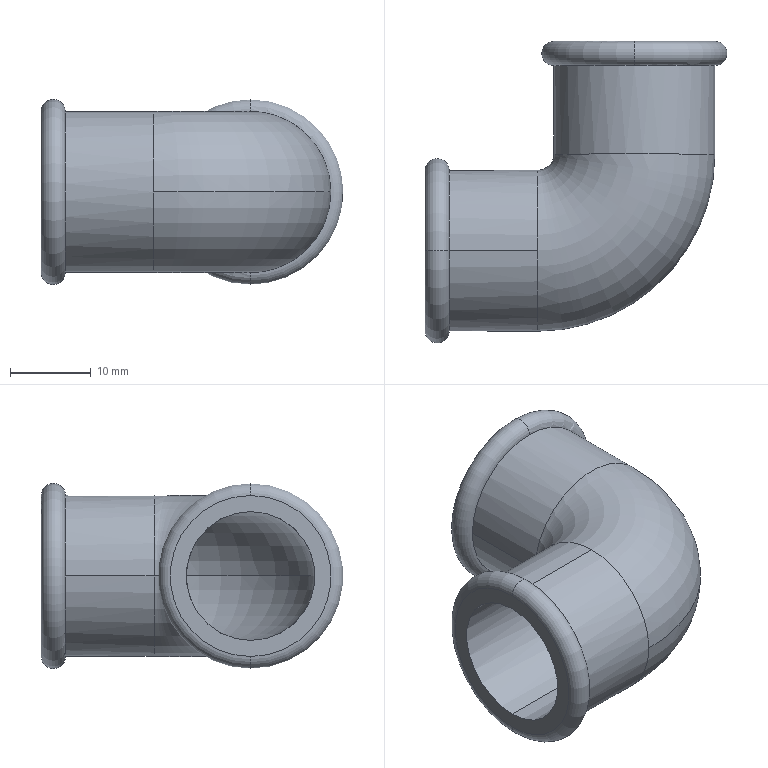Part | NX | features BREP 1 | 1 solid | 18 faces | box 37.5 x 37.5 x 23 mm | volume 5771 mm3 | torus 8 | cylinder 8 | plane 2 | commonest cylinder face diameters 16 x4 20 x4
STEP:
#1=CARTESIAN_POINT('',(34.,12.,0.));
#2=VERTEX_POINT('',#1);
#3=CARTESIAN_POINT('',(18.,12.,0.));
#4=VERTEX_POINT('',#3);
#5=CARTESIAN_POINT('',(26.,12.,0.));
#6=DIRECTION('',(0.,-1.,0.));
#7=DIRECTION('',(0.,0.,1.));
#8=AXIS2_PLACEMENT_3D('',#5,#6,#7);
#9=CIRCLE('',#8,8.);
#10=EDGE_CURVE('',#2,#4,#9,.T.);
#11=ORIENTED_EDGE('',*,*,#10,.F.);
#12=CARTESIAN_POINT('',(14.,-8.,0.));
#13=VERTEX_POINT('',#12);
#14=CARTESIAN_POINT('',(14.,12.,0.));
#15=DIRECTION('',(0.,0.,-1.));
#16=DIRECTION('',(-1.,0.,0.));
#17=AXIS2_PLACEMENT_3D('',#14,#15,#16);
#18=CIRCLE('',#17,20.);
#19=EDGE_CURVE('',#2,#13,#18,.T.);
#20=ORIENTED_EDGE('',*,*,#19,.T.);
#21=CARTESIAN_POINT('',(14.,0.,8.));
#22=VERTEX_POINT('',#21);
#23=CARTESIAN_POINT('',(14.,0.,0.));
#24=DIRECTION('',(-1.,0.,0.));
#25=DIRECTION('',(0.,0.,1.));
#26=AXIS2_PLACEMENT_3D('',#23,#24,#25);
#27=CIRCLE('',#26,8.);
#28=EDGE_CURVE('',#13,#22,#27,.T.);
#29=ORIENTED_EDGE('',*,*,#28,.T.);
#30=CARTESIAN_POINT('',(14.,8.,0.));
#31=VERTEX_POINT('',#30);
#32=CARTESIAN_POINT('',(14.,0.,0.));
#33=DIRECTION('',(-1.,0.,0.));
#34=DIRECTION('',(0.,0.,1.));
#35=AXIS2_PLACEMENT_3D('',#32,#33,#34);
#36=CIRCLE('',#35,8.);
#37=EDGE_CURVE('',#22,#31,#36,.T.);
#38=ORIENTED_EDGE('',*,*,#37,.T.);
#39=CARTESIAN_POINT('',(14.,12.,0.));
#40=DIRECTION('',(0.,0.,-1.));
#41=DIRECTION('',(-1.,0.,0.));
#42=AXIS2_PLACEMENT_3D('',#39,#40,#41);
#43=CIRCLE('',#42,4.);
#44=EDGE_CURVE('',#4,#31,#43,.T.);
#45=ORIENTED_EDGE('',*,*,#44,.F.);
#46=EDGE_LOOP('',(#11,#20,#29,#38,#45));
#47=FACE_BOUND('',#46,.T.);
#48=CARTESIAN_POINT('',(14.,12.,0.));
#49=DIRECTION('',(0.,0.,-1.));
#50=DIRECTION('',(-1.,0.,0.));
#51=AXIS2_PLACEMENT_3D('',#48,#49,#50);
#52=TOROIDAL_SURFACE('',#51,12.,8.);
#53=ADVANCED_FACE('',(#47),#52,.F.);
#54=CARTESIAN_POINT('',(16.,12.,0.));
#55=VERTEX_POINT('',#54);
#56=CARTESIAN_POINT('',(36.,12.,0.));
#57=VERTEX_POINT('',#56);
#58=CARTESIAN_POINT('',(26.,12.,0.));
#59=DIRECTION('',(0.,-1.,0.));
#60=DIRECTION('',(0.,0.,1.));
#61=AXIS2_PLACEMENT_3D('',#58,#59,#60);
#62=CIRCLE('',#61,10.);
#63=EDGE_CURVE('',#55,#57,#62,.T.);
#64=ORIENTED_EDGE('',*,*,#63,.T.);
#65=CARTESIAN_POINT('',(14.,-10.,0.));
#66=VERTEX_POINT('',#65);
#67=CARTESIAN_POINT('',(14.,12.,0.));
#68=DIRECTION('',(0.,0.,-1.));
#69=DIRECTION('',(-1.,0.,0.));
#70=AXIS2_PLACEMENT_3D('',#67,#68,#69);
#71=CIRCLE('',#70,22.);
#72=EDGE_CURVE('',#57,#66,#71,.T.);
#73=ORIENTED_EDGE('',*,*,#72,.T.);
#74=CARTESIAN_POINT('',(14.,0.,-10.));
#75=VERTEX_POINT('',#74);
#76=CARTESIAN_POINT('',(14.,0.,0.));
#77=DIRECTION('',(-1.,0.,0.));
#78=DIRECTION('',(0.,0.,1.));
#79=AXIS2_PLACEMENT_3D('',#76,#77,#78);
#80=CIRCLE('',#79,10.);
#81=EDGE_CURVE('',#75,#66,#80,.T.);
#82=ORIENTED_EDGE('',*,*,#81,.F.);
#83=CARTESIAN_POINT('',(14.,10.,0.));
#84=VERTEX_POINT('',#83);
#85=CARTESIAN_POINT('',(14.,0.,0.));
#86=DIRECTION('',(-1.,0.,0.));
#87=DIRECTION('',(0.,0.,1.));
#88=AXIS2_PLACEMENT_3D('',#85,#86,#87);
#89=CIRCLE('',#88,10.);
#90=EDGE_CURVE('',#84,#75,#89,.T.);
#91=ORIENTED_EDGE('',*,*,#90,.F.);
#92=CARTESIAN_POINT('',(14.,12.,0.));
#93=DIRECTION('',(0.,0.,-1.));
#94=DIRECTION('',(-1.,0.,0.));
#95=AXIS2_PLACEMENT_3D('',#92,#93,#94);
#96=CIRCLE('',#95,2.);
#97=EDGE_CURVE('',#55,#84,#96,.T.);
#98=ORIENTED_EDGE('',*,*,#97,.F.);
#99=EDGE_LOOP('',(#64,#73,#82,#91,#98));
#100=FACE_BOUND('',#99,.T.);
#101=CARTESIAN_POINT('',(14.,12.,0.));
#102=DIRECTION('',(0.,0.,-1.));
#103=DIRECTION('',(-1.,0.,0.));
#104=AXIS2_PLACEMENT_3D('',#101,#102,#103);
#105=TOROIDAL_SURFACE('',#104,12.,10.);
#106=ADVANCED_FACE('',(#100),#105,.T.);
#107=CARTESIAN_POINT('',(26.,26.,-10.));
#108=VERTEX_POINT('',#107);
#109=CARTESIAN_POINT('',(26.,26.,10.));
#110=VERTEX_POINT('',#109);
#111=CARTESIAN_POINT('',(26.,26.,0.));
#112=DIRECTION('',(0.,1.,0.));
#113=DIRECTION('',(0.,0.,1.));
#114=AXIS2_PLACEMENT_3D('',#111,#112,#113);
#115=CIRCLE('',#114,10.);
#116=EDGE_CURVE('',#108,#110,#115,.T.);
#117=ORIENTED_EDGE('',*,*,#116,.F.);
#118=CARTESIAN_POINT('',(26.,23.,-10.));
#119=VERTEX_POINT('',#118);
#120=CARTESIAN_POINT('',(26.,24.5,-10.));
#121=DIRECTION('',(-1.,0.,0.));
#122=DIRECTION('',(0.,0.,1.));
#123=AXIS2_PLACEMENT_3D('',#120,#121,#122);
#124=CIRCLE('',#123,1.5);
#125=EDGE_CURVE('',#108,#119,#124,.T.);
#126=ORIENTED_EDGE('',*,*,#125,.T.);
#127=CARTESIAN_POINT('',(16.,23.,0.));
#128=VERTEX_POINT('',#127);
#129=CARTESIAN_POINT('',(26.,23.,0.));
#130=DIRECTION('',(0.,1.,0.));
#131=DIRECTION('',(0.,0.,1.));
#132=AXIS2_PLACEMENT_3D('',#129,#130,#131);
#133=CIRCLE('',#132,10.);
#134=EDGE_CURVE('',#119,#128,#133,.T.);
#135=ORIENTED_EDGE('',*,*,#134,.T.);
#136=CARTESIAN_POINT('',(26.,23.,10.));
#137=VERTEX_POINT('',#136);
#138=CARTESIAN_POINT('',(26.,23.,0.));
#139=DIRECTION('',(0.,1.,0.));
#140=DIRECTION('',(0.,0.,1.));
#141=AXIS2_PLACEMENT_3D('',#138,#139,#140);
#142=CIRCLE('',#141,10.);
#143=EDGE_CURVE('',#128,#137,#142,.T.);
#144=ORIENTED_EDGE('',*,*,#143,.T.);
#145=CARTESIAN_POINT('',(26.,24.5,10.));
#146=DIRECTION('',(1.,0.,0.));
#147=DIRECTION('',(0.,0.,-1.));
#148=AXIS2_PLACEMENT_3D('',#145,#146,#147);
#149=CIRCLE('',#148,1.5);
#150=EDGE_CURVE('',#110,#137,#149,.T.);
#151=ORIENTED_EDGE('',*,*,#150,.F.);
#152=EDGE_LOOP('',(#117,#126,#135,#144,#151));
#153=FACE_BOUND('',#152,.T.);
#154=CARTESIAN_POINT('',(26.,24.5,0.));
#155=DIRECTION('',(0.,-1.,0.));
#156=DIRECTION('',(0.,0.,-1.));
#157=AXIS2_PLACEMENT_3D('',#154,#155,#156);
#158=TOROIDAL_SURFACE('',#157,10.,1.5);
#159=ADVANCED_FACE('',(#153),#158,.T.);
#160=CARTESIAN_POINT('',(3.,0.,10.));
#161=VERTEX_POINT('',#160);
#162=CARTESIAN_POINT('',(3.,0.,-10.));
#163=VERTEX_POINT('',#162);
#164=CARTESIAN_POINT('',(3.,0.,0.));
#165=DIRECTION('',(1.,0.,0.));
#166=DIRECTION('',(0.,0.,-1.));
#167=AXIS2_PLACEMENT_3D('',#164,#165,#166);
#168=CIRCLE('',#167,10.);
#169=EDGE_CURVE('',#161,#163,#168,.T.);
#170=ORIENTED_EDGE('',*,*,#169,.F.);
#171=CARTESIAN_POINT('',(0.,0.,10.));
#172=VERTEX_POINT('',#171);
#173=CARTESIAN_POINT('',(1.5,0.,10.));
#174=DIRECTION('',(0.,-1.,0.));
#175=DIRECTION('',(1.,0.,0.));
#176=AXIS2_PLACEMENT_3D('',#173,#174,#175);
#177=CIRCLE('',#176,1.5);
#178=EDGE_CURVE('',#172,#161,#177,.F.);
#179=ORIENTED_EDGE('',*,*,#178,.F.);
#180=CARTESIAN_POINT('',(0.,0.,-10.));
#181=VERTEX_POINT('',#180);
#182=CARTESIAN_POINT('',(0.,0.,0.));
#183=DIRECTION('',(-1.,0.,0.));
#184=DIRECTION('',(0.,0.,1.));
#185=AXIS2_PLACEMENT_3D('',#182,#183,#184);
#186=CIRCLE('',#185,10.);
#187=EDGE_CURVE('',#181,#172,#186,.T.);
#188=ORIENTED_EDGE('',*,*,#187,.F.);
#189=CARTESIAN_POINT('',(1.5,0.,-10.));
#190=DIRECTION('',(0.,1.,0.));
#191=DIRECTION('',(0.,0.,1.));
#192=AXIS2_PLACEMENT_3D('',#189,#190,#191);
#193=CIRCLE('',#192,1.5);
#194=EDGE_CURVE('',#181,#163,#193,.F.);
#195=ORIENTED_EDGE('',*,*,#194,.T.);
#196=EDGE_LOOP('',(#170,#179,#188,#195));
#197=FACE_BOUND('',#196,.T.);
#198=CARTESIAN_POINT('',(1.5,0.,0.));
#199=DIRECTION('',(-1.,0.,0.));
#200=DIRECTION('',(0.,0.,1.));
#201=AXIS2_PLACEMENT_3D('',#198,#199,#200);
#202=TOROIDAL_SURFACE('',#201,10.,1.5);
#203=ADVANCED_FACE('',(#197),#202,.T.);
#204=ORIENTED_EDGE('',*,*,#37,.F.);
#205=CARTESIAN_POINT('',(0.,0.,8.));
#206=VERTEX_POINT('',#205);
#207=CARTESIAN_POINT('',(14.,0.,8.));
#208=DIRECTION('',(-1.,0.,0.));
#209=VECTOR('',#208,1000.);
#210=LINE('',#207,#209);
#211=EDGE_CURVE('',#206,#22,#210,.F.);
#212=ORIENTED_EDGE('',*,*,#211,.F.);
#213=CARTESIAN_POINT('',(0.,0.,-8.));
#214=VERTEX_POINT('',#213);
#215=CARTESIAN_POINT('',(0.,0.,0.));
#216=DIRECTION('',(-1.,0.,0.));
#217=DIRECTION('',(0.,0.,1.));
#218=AXIS2_PLACEMENT_3D('',#215,#216,#217);
#219=CIRCLE('',#218,8.);
#220=EDGE_CURVE('',#206,#214,#219,.T.);
#221=ORIENTED_EDGE('',*,*,#220,.T.);
#222=CARTESIAN_POINT('',(14.,0.,-8.));
#223=VERTEX_POINT('',#222);
#224=CARTESIAN_POINT('',(14.,0.,-8.));
#225=DIRECTION('',(-1.,0.,0.));
#226=VECTOR('',#225,1000.);
#227=LINE('',#224,#226);
#228=EDGE_CURVE('',#214,#223,#227,.F.);
#229=ORIENTED_EDGE('',*,*,#228,.T.);
#230=CARTESIAN_POINT('',(14.,0.,0.));
#231=DIRECTION('',(-1.,0.,0.));
#232=DIRECTION('',(0.,0.,1.));
#233=AXIS2_PLACEMENT_3D('',#230,#231,#232);
#234=CIRCLE('',#233,8.);
#235=EDGE_CURVE('',#31,#223,#234,.T.);
#236=ORIENTED_EDGE('',*,*,#235,.F.);
#237=EDGE_LOOP('',(#204,#212,#221,#229,#236));
#238=FACE_BOUND('',#237,.T.);
#239=CARTESIAN_POINT('',(14.,0.,0.));
#240=DIRECTION('',(-1.,0.,0.));
#241=DIRECTION('',(0.,0.,1.));
#242=AXIS2_PLACEMENT_3D('',#239,#240,#241);
#243=CYLINDRICAL_SURFACE('',#242,8.);
#244=ADVANCED_FACE('',(#238),#243,.F.);
#245=CARTESIAN_POINT('',(26.,12.,0.));
#246=DIRECTION('',(0.,-1.,0.));
#247=DIRECTION('',(0.,0.,1.));
#248=AXIS2_PLACEMENT_3D('',#245,#246,#247);
#249=CIRCLE('',#248,8.);
#250=EDGE_CURVE('',#4,#2,#249,.T.);
#251=ORIENTED_EDGE('',*,*,#250,.T.);
#252=CARTESIAN_POINT('',(34.,26.,0.));
#253=VERTEX_POINT('',#252);
#254=CARTESIAN_POINT('',(34.,12.,0.));
#255=DIRECTION('',(0.,1.,0.));
#256=VECTOR('',#255,1000.);
#257=LINE('',#254,#256);
#258=EDGE_CURVE('',#253,#2,#257,.F.);
#259=ORIENTED_EDGE('',*,*,#258,.F.);
#260=CARTESIAN_POINT('',(18.,26.,0.));
#261=VERTEX_POINT('',#260);
#262=CARTESIAN_POINT('',(26.,26.,0.));
#263=DIRECTION('',(0.,-1.,0.));
#264=DIRECTION('',(0.,0.,1.));
#265=AXIS2_PLACEMENT_3D('',#262,#263,#264);
#266=CIRCLE('',#265,8.);
#267=EDGE_CURVE('',#261,#253,#266,.T.);
#268=ORIENTED_EDGE('',*,*,#267,.F.);
#269=CARTESIAN_POINT('',(18.,12.,0.));
#270=DIRECTION('',(0.,1.,0.));
#271=VECTOR('',#270,1000.);
#272=LINE('',#269,#271);
#273=EDGE_CURVE('',#261,#4,#272,.F.);
#274=ORIENTED_EDGE('',*,*,#273,.T.);
#275=EDGE_LOOP('',(#251,#259,#268,#274));
#276=FACE_BOUND('',#275,.T.);
#277=CARTESIAN_POINT('',(26.,12.,0.));
#278=DIRECTION('',(0.,1.,0.));
#279=DIRECTION('',(1.,0.,0.));
#280=AXIS2_PLACEMENT_3D('',#277,#278,#279);
#281=CYLINDRICAL_SURFACE('',#280,8.);
#282=ADVANCED_FACE('',(#276),#281,.F.);
#283=ORIENTED_EDGE('',*,*,#81,.T.);
#284=CARTESIAN_POINT('',(14.,0.,10.));
#285=VERTEX_POINT('',#284);
#286=CARTESIAN_POINT('',(14.,0.,0.));
#287=DIRECTION('',(-1.,0.,0.));
#288=DIRECTION('',(0.,0.,1.));
#289=AXIS2_PLACEMENT_3D('',#286,#287,#288);
#290=CIRCLE('',#289,10.);
#291=EDGE_CURVE('',#66,#285,#290,.T.);
#292=ORIENTED_EDGE('',*,*,#291,.T.);
#293=CARTESIAN_POINT('',(14.,0.,10.));
#294=DIRECTION('',(-1.,0.,0.));
#295=VECTOR('',#294,1000.);
#296=LINE('',#293,#295);
#297=EDGE_CURVE('',#161,#285,#296,.F.);
#298=ORIENTED_EDGE('',*,*,#297,.F.);
#299=ORIENTED_EDGE('',*,*,#169,.T.);
#300=CARTESIAN_POINT('',(14.,0.,-10.));
#301=DIRECTION('',(-1.,0.,0.));
#302=VECTOR('',#301,1000.);
#303=LINE('',#300,#302);
#304=EDGE_CURVE('',#163,#75,#303,.F.);
#305=ORIENTED_EDGE('',*,*,#304,.T.);
#306=EDGE_LOOP('',(#283,#292,#298,#299,#305));
#307=FACE_BOUND('',#306,.T.);
#308=CARTESIAN_POINT('',(14.,0.,0.));
#309=DIRECTION('',(-1.,0.,0.));
#310=DIRECTION('',(0.,0.,1.));
#311=AXIS2_PLACEMENT_3D('',#308,#309,#310);
#312=CYLINDRICAL_SURFACE('',#311,10.);
#313=ADVANCED_FACE('',(#307),#312,.T.);
#314=CARTESIAN_POINT('',(26.,12.,0.));
#315=DIRECTION('',(0.,-1.,0.));
#316=DIRECTION('',(0.,0.,1.));
#317=AXIS2_PLACEMENT_3D('',#314,#315,#316);
#318=CIRCLE('',#317,10.);
#319=EDGE_CURVE('',#57,#55,#318,.T.);
#320=ORIENTED_EDGE('',*,*,#319,.F.);
#321=CARTESIAN_POINT('',(36.,23.,0.));
#322=VERTEX_POINT('',#321);
#323=CARTESIAN_POINT('',(36.,12.,0.));
#324=DIRECTION('',(0.,1.,0.));
#325=VECTOR('',#324,1000.);
#326=LINE('',#323,#325);
#327=EDGE_CURVE('',#322,#57,#326,.F.);
#328=ORIENTED_EDGE('',*,*,#327,.F.);
#329=CARTESIAN_POINT('',(26.,23.,0.));
#330=DIRECTION('',(0.,1.,0.));
#331=DIRECTION('',(0.,0.,1.));
#332=AXIS2_PLACEMENT_3D('',#329,#330,#331);
#333=CIRCLE('',#332,10.);
#334=EDGE_CURVE('',#137,#322,#333,.T.);
#335=ORIENTED_EDGE('',*,*,#334,.F.);
#336=ORIENTED_EDGE('',*,*,#143,.F.);
#337=CARTESIAN_POINT('',(16.,12.,0.));
#338=DIRECTION('',(0.,1.,0.));
#339=VECTOR('',#338,1000.);
#340=LINE('',#337,#339);
#341=EDGE_CURVE('',#128,#55,#340,.F.);
#342=ORIENTED_EDGE('',*,*,#341,.T.);
#343=EDGE_LOOP('',(#320,#328,#335,#336,#342));
#344=FACE_BOUND('',#343,.T.);
#345=CARTESIAN_POINT('',(26.,12.,0.));
#346=DIRECTION('',(0.,1.,0.));
#347=DIRECTION('',(1.,0.,0.));
#348=AXIS2_PLACEMENT_3D('',#345,#346,#347);
#349=CYLINDRICAL_SURFACE('',#348,10.);
#350=ADVANCED_FACE('',(#344),#349,.T.);
#351=ORIENTED_EDGE('',*,*,#327,.T.);
#352=ORIENTED_EDGE('',*,*,#63,.F.);
#353=ORIENTED_EDGE('',*,*,#341,.F.);
#354=ORIENTED_EDGE('',*,*,#134,.F.);
#355=CARTESIAN_POINT('',(26.,23.,0.));
#356=DIRECTION('',(0.,1.,0.));
#357=DIRECTION('',(0.,0.,1.));
#358=AXIS2_PLACEMENT_3D('',#355,#356,#357);
#359=CIRCLE('',#358,10.);
#360=EDGE_CURVE('',#322,#119,#359,.T.);
#361=ORIENTED_EDGE('',*,*,#360,.F.);
#362=EDGE_LOOP('',(#351,#352,#353,#354,#361));
#363=FACE_BOUND('',#362,.T.);
#364=CARTESIAN_POINT('',(26.,12.,0.));
#365=DIRECTION('',(0.,1.,0.));
#366=DIRECTION('',(1.,0.,0.));
#367=AXIS2_PLACEMENT_3D('',#364,#365,#366);
#368=CYLINDRICAL_SURFACE('',#367,10.);
#369=ADVANCED_FACE('',(#363),#368,.T.);
#370=ORIENTED_EDGE('',*,*,#297,.T.);
#371=CARTESIAN_POINT('',(14.,0.,0.));
#372=DIRECTION('',(-1.,0.,0.));
#373=DIRECTION('',(0.,0.,1.));
#374=AXIS2_PLACEMENT_3D('',#371,#372,#373);
#375=CIRCLE('',#374,10.);
#376=EDGE_CURVE('',#285,#84,#375,.T.);
#377=ORIENTED_EDGE('',*,*,#376,.T.);
#378=ORIENTED_EDGE('',*,*,#90,.T.);
#379=ORIENTED_EDGE('',*,*,#304,.F.);
#380=CARTESIAN_POINT('',(3.,0.,0.));
#381=DIRECTION('',(1.,0.,0.));
#382=DIRECTION('',(0.,0.,-1.));
#383=AXIS2_PLACEMENT_3D('',#380,#381,#382);
#384=CIRCLE('',#383,10.);
#385=EDGE_CURVE('',#163,#161,#384,.T.);
#386=ORIENTED_EDGE('',*,*,#385,.T.);
#387=EDGE_LOOP('',(#370,#377,#378,#379,#386));
#388=FACE_BOUND('',#387,.T.);
#389=CARTESIAN_POINT('',(14.,0.,0.));
#390=DIRECTION('',(-1.,0.,0.));
#391=DIRECTION('',(0.,0.,1.));
#392=AXIS2_PLACEMENT_3D('',#389,#390,#391);
#393=CYLINDRICAL_SURFACE('',#392,10.);
#394=ADVANCED_FACE('',(#388),#393,.T.);
#395=ORIENTED_EDGE('',*,*,#258,.T.);
#396=ORIENTED_EDGE('',*,*,#10,.T.);
#397=ORIENTED_EDGE('',*,*,#273,.F.);
#398=CARTESIAN_POINT('',(26.,26.,0.));
#399=DIRECTION('',(0.,-1.,0.));
#400=DIRECTION('',(0.,0.,1.));
#401=AXIS2_PLACEMENT_3D('',#398,#399,#400);
#402=CIRCLE('',#401,8.);
#403=EDGE_CURVE('',#253,#261,#402,.T.);
#404=ORIENTED_EDGE('',*,*,#403,.F.);
#405=EDGE_LOOP('',(#395,#396,#397,#404));
#406=FACE_BOUND('',#405,.T.);
#407=CARTESIAN_POINT('',(26.,12.,0.));
#408=DIRECTION('',(0.,1.,0.));
#409=DIRECTION('',(1.,0.,0.));
#410=AXIS2_PLACEMENT_3D('',#407,#408,#409);
#411=CYLINDRICAL_SURFACE('',#410,8.);
#412=ADVANCED_FACE('',(#406),#411,.F.);
#413=ORIENTED_EDGE('',*,*,#72,.F.);
#414=ORIENTED_EDGE('',*,*,#319,.T.);
#415=ORIENTED_EDGE('',*,*,#97,.T.);
#416=ORIENTED_EDGE('',*,*,#376,.F.);
#417=ORIENTED_EDGE('',*,*,#291,.F.);
#418=EDGE_LOOP('',(#413,#414,#415,#416,#417));
#419=FACE_BOUND('',#418,.T.);
#420=CARTESIAN_POINT('',(14.,12.,0.));
#421=DIRECTION('',(0.,0.,-1.));
#422=DIRECTION('',(-1.,0.,0.));
#423=AXIS2_PLACEMENT_3D('',#420,#421,#422);
#424=TOROIDAL_SURFACE('',#423,12.,10.);
#425=ADVANCED_FACE('',(#419),#424,.T.);
#426=ORIENTED_EDGE('',*,*,#19,.F.);
#427=ORIENTED_EDGE('',*,*,#250,.F.);
#428=ORIENTED_EDGE('',*,*,#44,.T.);
#429=ORIENTED_EDGE('',*,*,#235,.T.);
#430=CARTESIAN_POINT('',(14.,0.,0.));
#431=DIRECTION('',(-1.,0.,0.));
#432=DIRECTION('',(0.,0.,1.));
#433=AXIS2_PLACEMENT_3D('',#430,#431,#432);
#434=CIRCLE('',#433,8.);
#435=EDGE_CURVE('',#223,#13,#434,.T.);
#436=ORIENTED_EDGE('',*,*,#435,.T.);
#437=EDGE_LOOP('',(#426,#427,#428,#429,#436));
#438=FACE_BOUND('',#437,.T.);
#439=CARTESIAN_POINT('',(14.,12.,0.));
#440=DIRECTION('',(0.,0.,-1.));
#441=DIRECTION('',(-1.,0.,0.));
#442=AXIS2_PLACEMENT_3D('',#439,#440,#441);
#443=TOROIDAL_SURFACE('',#442,12.,8.);
#444=ADVANCED_FACE('',(#438),#443,.F.);
#445=ORIENTED_EDGE('',*,*,#211,.T.);
#446=ORIENTED_EDGE('',*,*,#28,.F.);
#447=ORIENTED_EDGE('',*,*,#435,.F.);
#448=ORIENTED_EDGE('',*,*,#228,.F.);
#449=CARTESIAN_POINT('',(0.,0.,0.));
#450=DIRECTION('',(-1.,0.,0.));
#451=DIRECTION('',(0.,0.,1.));
#452=AXIS2_PLACEMENT_3D('',#449,#450,#451);
#453=CIRCLE('',#452,8.);
#454=EDGE_CURVE('',#214,#206,#453,.T.);
#455=ORIENTED_EDGE('',*,*,#454,.T.);
#456=EDGE_LOOP('',(#445,#446,#447,#448,#455));
#457=FACE_BOUND('',#456,.T.);
#458=CARTESIAN_POINT('',(14.,0.,0.));
#459=DIRECTION('',(-1.,0.,0.));
#460=DIRECTION('',(0.,0.,1.));
#461=AXIS2_PLACEMENT_3D('',#458,#459,#460);
#462=CYLINDRICAL_SURFACE('',#461,8.);
#463=ADVANCED_FACE('',(#457),#462,.F.);
#464=CARTESIAN_POINT('',(26.,26.,0.));
#465=DIRECTION('',(0.,1.,0.));
#466=DIRECTION('',(0.,0.,1.));
#467=AXIS2_PLACEMENT_3D('',#464,#465,#466);
#468=CIRCLE('',#467,10.);
#469=EDGE_CURVE('',#110,#108,#468,.T.);
#470=ORIENTED_EDGE('',*,*,#469,.T.);
#471=ORIENTED_EDGE('',*,*,#116,.T.);
#472=EDGE_LOOP('',(#470,#471));
#473=FACE_BOUND('',#472,.T.);
#474=ORIENTED_EDGE('',*,*,#267,.T.);
#475=ORIENTED_EDGE('',*,*,#403,.T.);
#476=EDGE_LOOP('',(#474,#475));
#477=FACE_BOUND('',#476,.T.);
#478=CARTESIAN_POINT('',(26.,26.,0.));
#479=DIRECTION('',(0.,1.,0.));
#480=DIRECTION('',(0.,0.,1.));
#481=AXIS2_PLACEMENT_3D('',#478,#479,#480);
#482=PLANE('',#481);
#483=ADVANCED_FACE('',(#473,#477),#482,.T.);
#484=ORIENTED_EDGE('',*,*,#187,.T.);
#485=CARTESIAN_POINT('',(0.,0.,0.));
#486=DIRECTION('',(-1.,0.,0.));
#487=DIRECTION('',(0.,0.,1.));
#488=AXIS2_PLACEMENT_3D('',#485,#486,#487);
#489=CIRCLE('',#488,10.);
#490=EDGE_CURVE('',#172,#181,#489,.T.);
#491=ORIENTED_EDGE('',*,*,#490,.T.);
#492=EDGE_LOOP('',(#484,#491));
#493=FACE_BOUND('',#492,.T.);
#494=ORIENTED_EDGE('',*,*,#454,.F.);
#495=ORIENTED_EDGE('',*,*,#220,.F.);
#496=EDGE_LOOP('',(#494,#495));
#497=FACE_BOUND('',#496,.T.);
#498=CARTESIAN_POINT('',(0.,0.,0.));
#499=DIRECTION('',(1.,0.,0.));
#500=DIRECTION('',(0.,0.,-1.));
#501=AXIS2_PLACEMENT_3D('',#498,#499,#500);
#502=PLANE('',#501);
#503=ADVANCED_FACE('',(#493,#497),#502,.F.);
#504=ORIENTED_EDGE('',*,*,#178,.T.);
#505=ORIENTED_EDGE('',*,*,#385,.F.);
#506=ORIENTED_EDGE('',*,*,#194,.F.);
#507=ORIENTED_EDGE('',*,*,#490,.F.);
#508=EDGE_LOOP('',(#504,#505,#506,#507));
#509=FACE_BOUND('',#508,.T.);
#510=CARTESIAN_POINT('',(1.5,0.,0.));
#511=DIRECTION('',(-1.,0.,0.));
#512=DIRECTION('',(0.,0.,1.));
#513=AXIS2_PLACEMENT_3D('',#510,#511,#512);
#514=TOROIDAL_SURFACE('',#513,10.,1.5);
#515=ADVANCED_FACE('',(#509),#514,.T.);
#516=ORIENTED_EDGE('',*,*,#125,.F.);
#517=ORIENTED_EDGE('',*,*,#469,.F.);
#518=ORIENTED_EDGE('',*,*,#150,.T.);
#519=ORIENTED_EDGE('',*,*,#334,.T.);
#520=ORIENTED_EDGE('',*,*,#360,.T.);
#521=EDGE_LOOP('',(#516,#517,#518,#519,#520));
#522=FACE_BOUND('',#521,.T.);
#523=CARTESIAN_POINT('',(26.,24.5,0.));
#524=DIRECTION('',(0.,-1.,0.));
#525=DIRECTION('',(0.,0.,-1.));
#526=AXIS2_PLACEMENT_3D('',#523,#524,#525);
#527=TOROIDAL_SURFACE('',#526,10.,1.5);
#528=ADVANCED_FACE('',(#522),#527,.T.);
#529=CLOSED_SHELL('',(#53,#106,#159,#203,#244,#282,#313,#350,#369,#394,#412,#425,#444,#463,#483,#503,#515,#528));
#530=MANIFOLD_SOLID_BREP('',#529);
#531=(LENGTH_UNIT()NAMED_UNIT(*)SI_UNIT(.MILLI.,.METRE.));
#532=UNCERTAINTY_MEASURE_WITH_UNIT(LENGTH_MEASURE(0.00001),#531,'','');
#533=(NAMED_UNIT(*)PLANE_ANGLE_UNIT()SI_UNIT($,.RADIAN.));
#534=(NAMED_UNIT(*)SI_UNIT($,.STERADIAN.)SOLID_ANGLE_UNIT());
#535=(GEOMETRIC_REPRESENTATION_CONTEXT(3)GLOBAL_UNCERTAINTY_ASSIGNED_CONTEXT((#532))GLOBAL_UNIT_ASSIGNED_CONTEXT((#531,#533,#534))REPRESENTATION_CONTEXT('',''));
#536=ADVANCED_BREP_SHAPE_REPRESENTATION('',(#530),#535);